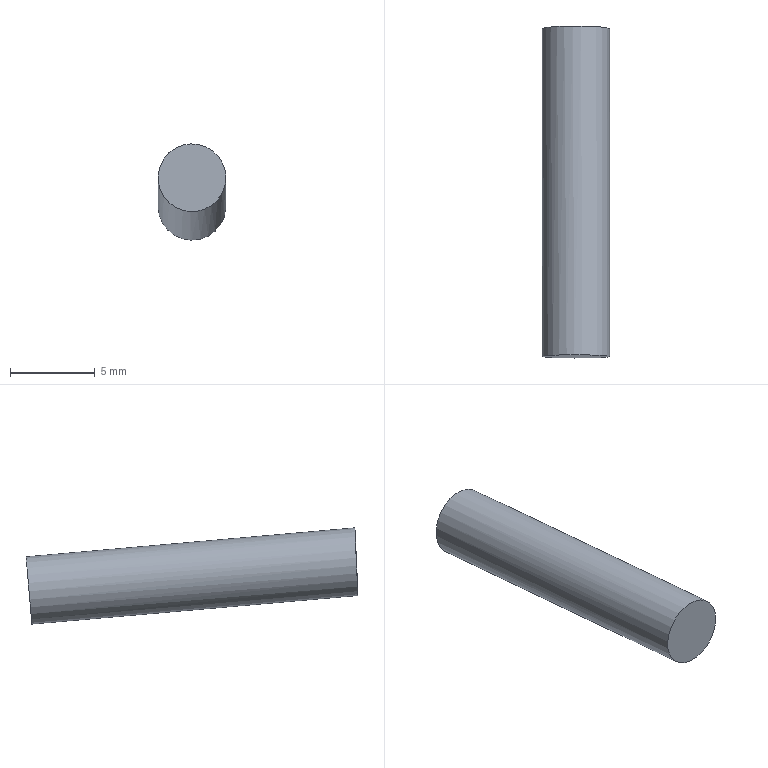Part | NX | features solid 2 | 1 solid | 3 faces | box 4 x 19.589 x 5.683 mm | volume 243.754 mm3 | plane 2 | cylinder 1 | commonest cylinder face diameters 4 x1
STEP:
#1=CARTESIAN_POINT('',(118.936,-26.625,-31.021));
#2=VERTEX_POINT('',#1);
#3=CARTESIAN_POINT('',(118.936,-26.451,-29.029));
#4=DIRECTION('',(0.,-0.9962,0.08716));
#5=DIRECTION('',(0.,-0.08716,-0.9962));
#6=AXIS2_PLACEMENT_3D('',#3,#4,#5);
#7=CIRCLE('',#6,2.);
#8=EDGE_CURVE('',#2,#2,#7,.T.);
#9=ORIENTED_EDGE('',*,*,#8,.F.);
#10=EDGE_LOOP('',(#9));
#11=FACE_BOUND('',#10,.T.);
#12=CARTESIAN_POINT('',(118.936,-26.451,-29.029));
#13=DIRECTION('',(0.,0.9962,-0.08716));
#14=DIRECTION('',(0.,0.08716,0.9962));
#15=AXIS2_PLACEMENT_3D('',#12,#13,#14);
#16=PLANE('',#15);
#17=ADVANCED_FACE('',(#11),#16,.T.);
#18=CARTESIAN_POINT('',(118.843,-45.865,-29.336));
#19=VERTEX_POINT('',#18);
#20=CARTESIAN_POINT('',(118.936,-45.774,-27.338));
#21=DIRECTION('',(0.001957,0.999,-0.04546));
#22=DIRECTION('',(-0.04675,-0.04532,-0.9979));
#23=AXIS2_PLACEMENT_3D('',#20,#21,#22);
#24=ELLIPSE('',#23,2.002,2.);
#25=EDGE_CURVE('',#19,#19,#24,.T.);
#26=ORIENTED_EDGE('',*,*,#25,.F.);
#27=EDGE_LOOP('',(#26));
#28=FACE_BOUND('',#27,.T.);
#29=CARTESIAN_POINT('',(128.811,-48.589,-88.763));
#30=DIRECTION('',(0.001957,0.999,-0.04546));
#31=DIRECTION('',(0.06617,0.04523,0.9968));
#32=AXIS2_PLACEMENT_3D('',#29,#30,#31);
#33=PLANE('',#32);
#34=ADVANCED_FACE('',(#28),#33,.F.);
#35=ORIENTED_EDGE('',*,*,#8,.T.);
#36=EDGE_LOOP('',(#35));
#37=FACE_BOUND('',#36,.T.);
#38=ORIENTED_EDGE('',*,*,#25,.T.);
#39=EDGE_LOOP('',(#38));
#40=FACE_BOUND('',#39,.T.);
#41=CARTESIAN_POINT('',(118.936,-46.375,-27.286));
#42=DIRECTION('',(0.,0.9962,-0.08716));
#43=DIRECTION('',(0.,0.08716,0.9962));
#44=AXIS2_PLACEMENT_3D('',#41,#42,#43);
#45=CYLINDRICAL_SURFACE('',#44,2.);
#46=ADVANCED_FACE('',(#37,#40),#45,.T.);
#47=CLOSED_SHELL('',(#17,#34,#46));
#48=MANIFOLD_SOLID_BREP('',#47);
#49=(LENGTH_UNIT()NAMED_UNIT(*)SI_UNIT(.MILLI.,.METRE.));
#50=UNCERTAINTY_MEASURE_WITH_UNIT(LENGTH_MEASURE(0.00001),#49,'','');
#51=(NAMED_UNIT(*)PLANE_ANGLE_UNIT()SI_UNIT($,.RADIAN.));
#52=(NAMED_UNIT(*)SI_UNIT($,.STERADIAN.)SOLID_ANGLE_UNIT());
#53=(GEOMETRIC_REPRESENTATION_CONTEXT(3)GLOBAL_UNCERTAINTY_ASSIGNED_CONTEXT((#50))GLOBAL_UNIT_ASSIGNED_CONTEXT((#49,#51,#52))REPRESENTATION_CONTEXT('',''));
#54=ADVANCED_BREP_SHAPE_REPRESENTATION('',(#48),#53);